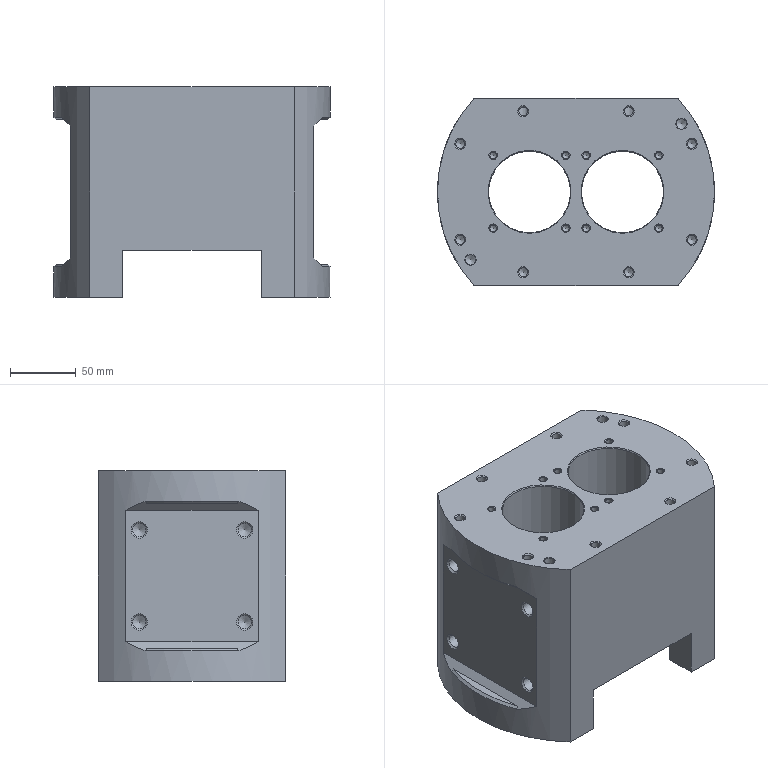NC program | NX | posted with a generic post | part box 210 x 142 x 160 mm
Lines 1 to 1156 of 4199:
N10 G17 G21 G94 G90
(FLOOR_WALL_COPY_COPY_COPY_COPY_1_COPY , TOOL : D50)
N12 T02 M6
N14 G54
N16 G17 G0 G90 X-133. Y70.997 B0. C0. S2500 M3
N18 G43 Z30. H2
N20 Z3.
N22 G94 G1 Z0. F1000.
N24 X-130.
N26 X130.
N28 Y40.498
N30 X-130.
N32 Y9.999
N34 X130.
N36 Y-20.501
N38 X-130.
N40 Y-51.
N42 X130.
N44 X133.
N46 Z3.
N48 G0 Z30.
(FLOOR_WALL_1 , TOOL : D50)
N50 X3.83 Y-99. S1200
N52 Z0.652
N54 G1 Z-0.348
N56 Y-72.786
N58 G3 X0. Y-71. R5.
N60 G1 X-27.35 F2000.
N62 Y-30.308
N64 X-43.993 Y-24.326
N66 G2 X-43.993 Y24.326 R25.85
N68 G1 X-33.127 Y28.232
N70 X-27.35 Y30.308
N72 Y71.
N74 X27.35
N76 Y30.308
N78 X43.993 Y24.326
N80 G2 X43.993 Y-24.326 R25.85
N82 G1 X33.127 Y-28.232
N84 X27.35 Y-30.308
N86 Y-71.
N88 X0.
N90 Y-17.98
N92 G3 X-17.203 Y-2.077 R30.
N94 G1 X-22.98 Y0.
N96 X-17.204 Y2.076
N98 G3 X0. Y17.98 R30.
N100 G1 Y44.472
N102 Y17.98
N104 G3 X17.203 Y2.077 R30.
N106 G1 X22.98 Y0.
N108 X17.203 Y-2.077
N110 G3 X0. Y-17.98 R30.
N112 X0.054 Y-22.206 R5.
N114 G1 Z0.652
N116 G0 X3.83 Y-99. Z0.304
N118 G1 Z-0.696 F1000.
N120 Y-72.786
N122 G3 X0. Y-71. R5.
N124 G1 X-27.35 F2000.
N126 Y-30.308
N128 X-43.993 Y-24.326
N130 G2 X-43.993 Y24.326 R25.85
N132 G1 X-33.127 Y28.232
N134 X-27.35 Y30.308
N136 Y71.
N138 X27.35
N140 Y30.308
N142 X43.993 Y24.326
N144 G2 X43.993 Y-24.326 R25.85
N146 G1 X33.127 Y-28.232
N148 X27.35 Y-30.308
N150 Y-71.
N152 X0.
N154 Y-17.98
N156 G3 X-17.203 Y-2.077 R30.
N158 G1 X-22.98 Y0.
N160 X-17.204 Y2.076
N162 G3 X0. Y17.98 R30.
N164 G1 Y44.472
N166 Y17.98
N168 G3 X17.203 Y2.077 R30.
N170 G1 X22.98 Y0.
N172 X17.203 Y-2.077
N174 G3 X0. Y-17.98 R30.
N176 X0.054 Y-22.206 R5.
N178 G1 Z0.304
N180 G0 X3.83 Y-99. Z-0.044
N182 G1 Z-1.044 F1000.
N184 Y-72.786
N186 G3 X0. Y-71. R5.
N188 G1 X-27.35 F2000.
N190 Y-30.308
N192 X-43.993 Y-24.326
N194 G2 X-43.993 Y24.326 R25.85
N196 G1 X-33.127 Y28.232
N198 X-27.35 Y30.308
N200 Y71.
N202 X27.35
N204 Y30.308
N206 X43.993 Y24.326
N208 G2 X43.993 Y-24.326 R25.85
N210 G1 X33.127 Y-28.232
N212 X27.35 Y-30.308
N214 Y-71.
N216 X0.
N218 Y-17.98
N220 G3 X-17.203 Y-2.077 R30.
N222 G1 X-22.98 Y0.
N224 X-17.204 Y2.076
N226 G3 X0. Y17.98 R30.
N228 G1 Y44.472
N230 Y17.98
N232 G3 X17.203 Y2.077 R30.
N234 G1 X22.98 Y0.
N236 X17.203 Y-2.077
N238 G3 X0. Y-17.98 R30.
N240 X0.054 Y-22.206 R5.
N242 G1 Z-0.044
N244 G0 X3.83 Y-99. Z-0.392
N246 G1 Z-1.392 F1000.
N248 Y-72.786
N250 G3 X0. Y-71. R5.
N252 G1 X-27.35 F2000.
N254 Y-30.308
N256 X-43.993 Y-24.326
N258 G2 X-43.993 Y24.326 R25.85
N260 G1 X-33.127 Y28.232
N262 X-27.35 Y30.308
N264 Y71.
N266 X27.35
N268 Y30.308
N270 X43.993 Y24.326
N272 G2 X43.993 Y-24.326 R25.85
N274 G1 X33.127 Y-28.232
N276 X27.35 Y-30.308
N278 Y-71.
N280 X0.
N282 Y-17.98
N284 G3 X-17.203 Y-2.077 R30.
N286 G1 X-22.98 Y0.
N288 X-17.204 Y2.076
N290 G3 X0. Y17.98 R30.
N292 G1 Y44.472
N294 Y17.98
N296 G3 X17.203 Y2.077 R30.
N298 G1 X22.98 Y0.
N300 X17.203 Y-2.077
N302 G3 X0. Y-17.98 R30.
N304 X0.054 Y-22.206 R5.
N306 G1 Z-0.392
N308 G0 X3.83 Y-99. Z-0.74
N310 G1 Z-1.74 F1000.
N312 Y-72.786
N314 G3 X0. Y-71. R5.
N316 G1 X-27.35 F2000.
N318 Y-30.308
N320 X-43.993 Y-24.326
N322 G2 X-43.993 Y24.326 R25.85
N324 G1 X-33.127 Y28.232
N326 X-27.35 Y30.308
N328 Y71.
N330 X27.35
N332 Y30.308
N334 X43.993 Y24.326
N336 G2 X43.993 Y-24.326 R25.85
N338 G1 X33.127 Y-28.232
N340 X27.35 Y-30.308
N342 Y-71.
N344 X0.
N346 Y-17.98
N348 G3 X-17.203 Y-2.077 R30.
N350 G1 X-22.98 Y0.
N352 X-17.204 Y2.076
N354 G3 X0. Y17.98 R30.
N356 G1 Y44.472
N358 Y17.98
N360 G3 X17.203 Y2.077 R30.
N362 G1 X22.98 Y0.
N364 X17.203 Y-2.077
N366 G3 X0. Y-17.98 R30.
N368 X0.054 Y-22.206 R5.
N370 G1 Z-0.74
N372 G0 X3.83 Y-99. Z-1.088
N374 G1 Z-2.088 F1000.
N376 Y-72.786
N378 G3 X0. Y-71. R5.
N380 G1 X-27.35 F2000.
N382 Y-30.308
N384 X-43.993 Y-24.326
N386 G2 X-43.993 Y24.326 R25.85
N388 G1 X-33.127 Y28.232
N390 X-27.35 Y30.308
N392 Y71.
N394 X27.35
N396 Y30.308
N398 X43.993 Y24.326
N400 G2 X43.993 Y-24.326 R25.85
N402 G1 X33.127 Y-28.232
N404 X27.35 Y-30.308
N406 Y-71.
N408 X0.
N410 Y-17.98
N412 G3 X-17.203 Y-2.077 R30.
N414 G1 X-22.98 Y0.
N416 X-17.204 Y2.076
N418 G3 X0. Y17.98 R30.
N420 G1 Y44.472
N422 Y17.98
N424 G3 X17.203 Y2.077 R30.
N426 G1 X22.98 Y0.
N428 X17.203 Y-2.077
N430 G3 X0. Y-17.98 R30.
N432 X0.054 Y-22.206 R5.
N434 G1 Z-1.088
N436 G0 X3.83 Y-99. Z-1.436
N438 G1 Z-2.436 F1000.
N440 Y-72.786
N442 G3 X0. Y-71. R5.
N444 G1 X-27.35 F2000.
N446 Y-30.308
N448 X-43.993 Y-24.326
N450 G2 X-43.993 Y24.326 R25.85
N452 G1 X-33.127 Y28.232
N454 X-27.35 Y30.308
N456 Y71.
N458 X27.35
N460 Y30.308
N462 X43.993 Y24.326
N464 G2 X43.993 Y-24.326 R25.85
N466 G1 X33.127 Y-28.232
N468 X27.35 Y-30.308
N470 Y-71.
N472 X0.
N474 Y-17.98
N476 G3 X-17.203 Y-2.077 R30.
N478 G1 X-22.98 Y0.
N480 X-17.204 Y2.076
N482 G3 X0. Y17.98 R30.
N484 G1 Y44.472
N486 Y17.98
N488 G3 X17.203 Y2.077 R30.
N490 G1 X22.98 Y0.
N492 X17.203 Y-2.077
N494 G3 X0. Y-17.98 R30.
N496 X0.054 Y-22.206 R5.
N498 G1 Z-1.436
N500 G0 X3.83 Y-99. Z-1.784
N502 G1 Z-2.784 F1000.
N504 Y-72.786
N506 G3 X0. Y-71. R5.
N508 G1 X-27.35 F2000.
N510 Y-30.308
N512 X-43.993 Y-24.326
N514 G2 X-43.993 Y24.326 R25.85
N516 G1 X-33.127 Y28.232
N518 X-27.35 Y30.308
N520 Y71.
N522 X27.35
N524 Y30.308
N526 X43.993 Y24.326
N528 G2 X43.993 Y-24.326 R25.85
N530 G1 X33.127 Y-28.232
N532 X27.35 Y-30.308
N534 Y-71.
N536 X0.
N538 Y-17.98
N540 G3 X-17.203 Y-2.077 R30.
N542 G1 X-22.98 Y0.
N544 X-17.204 Y2.076
N546 G3 X0. Y17.98 R30.
N548 G1 Y44.472
N550 Y17.98
N552 G3 X17.203 Y2.077 R30.
N554 G1 X22.98 Y0.
N556 X17.203 Y-2.077
N558 G3 X0. Y-17.98 R30.
N560 X0.054 Y-22.206 R5.
N562 G1 Z-1.784
N564 G0 X3.83 Y-99. Z-2.133
N566 G1 Z-3.133 F1000.
N568 Y-72.786
N570 G3 X0. Y-71. R5.
N572 G1 X-27.35 F2000.
N574 Y-30.308
N576 X-43.993 Y-24.326
N578 G2 X-43.993 Y24.326 R25.85
N580 G1 X-33.127 Y28.232
N582 X-27.35 Y30.308
N584 Y71.
N586 X27.35
N588 Y30.308
N590 X43.993 Y24.326
N592 G2 X43.993 Y-24.326 R25.85
N594 G1 X33.127 Y-28.232
N596 X27.35 Y-30.308
N598 Y-71.
N600 X0.
N602 Y-17.98
N604 G3 X-17.203 Y-2.077 R30.
N606 G1 X-22.98 Y0.
N608 X-17.204 Y2.076
N610 G3 X0. Y17.98 R30.
N612 G1 Y44.472
N614 Y17.98
N616 G3 X17.203 Y2.077 R30.
N618 G1 X22.98 Y0.
N620 X17.203 Y-2.077
N622 G3 X0. Y-17.98 R30.
N624 X0.054 Y-22.206 R5.
N626 G1 Z-2.133
N628 G0 X3.83 Y-99. Z-2.481
N630 G1 Z-3.481 F1000.
N632 Y-72.786
N634 G3 X0. Y-71. R5.
N636 G1 X-27.35 F2000.
N638 Y-30.308
N640 X-43.993 Y-24.326
N642 G2 X-43.993 Y24.326 R25.85
N644 G1 X-33.127 Y28.232
N646 X-27.35 Y30.308
N648 Y71.
N650 X27.35
N652 Y30.308
N654 X43.993 Y24.326
N656 G2 X43.993 Y-24.326 R25.85
N658 G1 X33.127 Y-28.232
N660 X27.35 Y-30.308
N662 Y-71.
N664 X0.
N666 Y-17.98
N668 G3 X-17.203 Y-2.077 R30.
N670 G1 X-22.98 Y0.
N672 X-17.204 Y2.076
N674 G3 X0. Y17.98 R30.
N676 G1 Y44.472
N678 Y17.98
N680 G3 X17.203 Y2.077 R30.
N682 G1 X22.98 Y0.
N684 X17.203 Y-2.077
N686 G3 X0. Y-17.98 R30.
N688 X0.054 Y-22.206 R5.
N690 G1 Z-2.481
N692 G0 X3.83 Y-99. Z-2.829
N694 G1 Z-3.829 F1000.
N696 Y-72.786
N698 G3 X0. Y-71. R5.
N700 G1 X-27.35 F2000.
N702 Y-30.308
N704 X-43.993 Y-24.326
N706 G2 X-43.993 Y24.326 R25.85
N708 G1 X-33.127 Y28.232
N710 X-27.35 Y30.308
N712 Y71.
N714 X27.35
N716 Y30.308
N718 X43.993 Y24.326
N720 G2 X43.993 Y-24.326 R25.85
N722 G1 X33.127 Y-28.232
N724 X27.35 Y-30.308
N726 Y-71.
N728 X0.
N730 Y-17.98
N732 G3 X-17.203 Y-2.077 R30.
N734 G1 X-22.98 Y0.
N736 X-17.204 Y2.076
N738 G3 X0. Y17.98 R30.
N740 G1 Y44.472
N742 Y17.98
N744 G3 X17.203 Y2.077 R30.
N746 G1 X22.98 Y0.
N748 X17.203 Y-2.077
N750 G3 X0. Y-17.98 R30.
N752 X0.054 Y-22.206 R5.
N754 G1 Z-2.829
N756 G0 X3.83 Y-99. Z-3.177
N758 G1 Z-4.177 F1000.
N760 Y-72.786
N762 G3 X0. Y-71. R5.
N764 G1 X-27.35 F2000.
N766 Y-30.308
N768 X-43.993 Y-24.326
N770 G2 X-43.993 Y24.326 R25.85
N772 G1 X-33.127 Y28.232
N774 X-27.35 Y30.308
N776 Y71.
N778 X27.35
N780 Y30.308
N782 X43.993 Y24.326
N784 G2 X43.993 Y-24.326 R25.85
N786 G1 X33.127 Y-28.232
N788 X27.35 Y-30.308
N790 Y-71.
N792 X0.
N794 Y-17.98
N796 G3 X-17.203 Y-2.077 R30.
N798 G1 X-22.98 Y0.
N800 X-17.204 Y2.076
N802 G3 X0. Y17.98 R30.
N804 G1 Y44.472
N806 Y17.98
N808 G3 X17.203 Y2.077 R30.
N810 G1 X22.98 Y0.
N812 X17.203 Y-2.077
N814 G3 X0. Y-17.98 R30.
N816 X0.054 Y-22.206 R5.
N818 G1 Z-3.177
N820 G0 X3.83 Y-99. Z-3.525
N822 G1 Z-4.525 F1000.
N824 Y-72.786
N826 G3 X0. Y-71. R5.
N828 G1 X-27.35 F2000.
N830 Y-30.308
N832 X-43.993 Y-24.326
N834 G2 X-43.993 Y24.326 R25.85
N836 G1 X-33.127 Y28.232
N838 X-27.35 Y30.308
N840 Y71.
N842 X27.35
N844 Y30.308
N846 X43.993 Y24.326
N848 G2 X43.993 Y-24.326 R25.85
N850 G1 X33.127 Y-28.232
N852 X27.35 Y-30.308
N854 Y-71.
N856 X0.
N858 Y-17.98
N860 G3 X-17.203 Y-2.077 R30.
N862 G1 X-22.98 Y0.
N864 X-17.204 Y2.076
N866 G3 X0. Y17.98 R30.
N868 G1 Y44.472
N870 Y17.98
N872 G3 X17.203 Y2.077 R30.
N874 G1 X22.98 Y0.
N876 X17.203 Y-2.077
N878 G3 X0. Y-17.98 R30.
N880 X0.054 Y-22.206 R5.
N882 G1 Z-3.525
N884 G0 X3.83 Y-99. Z-3.873
N886 G1 Z-4.873 F1000.
N888 Y-72.786
N890 G3 X0. Y-71. R5.
N892 G1 X-27.35 F2000.
N894 Y-30.308
N896 X-43.993 Y-24.326
N898 G2 X-43.993 Y24.326 R25.85
N900 G1 X-33.127 Y28.232
N902 X-27.35 Y30.308
N904 Y71.
N906 X27.35
N908 Y30.308
N910 X43.993 Y24.326
N912 G2 X43.993 Y-24.326 R25.85
N914 G1 X33.127 Y-28.232
N916 X27.35 Y-30.308
N918 Y-71.
N920 X0.
N922 Y-17.98
N924 G3 X-17.203 Y-2.077 R30.
N926 G1 X-22.98 Y0.
N928 X-17.204 Y2.076
N930 G3 X0. Y17.98 R30.
N932 G1 Y44.472
N934 Y17.98
N936 G3 X17.203 Y2.077 R30.
N938 G1 X22.98 Y0.
N940 X17.203 Y-2.077
N942 G3 X0. Y-17.98 R30.
N944 X0.054 Y-22.206 R5.
N946 G1 Z-3.873
N948 G0 X3.83 Y-99. Z-4.221
N950 G1 Z-5.221 F1000.
N952 Y-72.786
N954 G3 X0. Y-71. R5.
N956 G1 X-27.35 F2000.
N958 Y-30.308
N960 X-43.993 Y-24.326
N962 G2 X-43.993 Y24.326 R25.85
N964 G1 X-33.127 Y28.232
N966 X-27.35 Y30.308
N968 Y71.
N970 X27.35
N972 Y30.308
N974 X43.993 Y24.326
N976 G2 X43.993 Y-24.326 R25.85
N978 G1 X33.127 Y-28.232
N980 X27.35 Y-30.308
N982 Y-71.
N984 X0.
N986 Y-17.98
N988 G3 X-17.203 Y-2.077 R30.
N990 G1 X-22.98 Y0.
N992 X-17.204 Y2.076
N994 G3 X0. Y17.98 R30.
N996 G1 Y44.472
N998 Y17.98
N1000 G3 X17.203 Y2.077 R30.
N1002 G1 X22.98 Y0.
N1004 X17.203 Y-2.077
N1006 G3 X0. Y-17.98 R30.
N1008 X0.054 Y-22.206 R5.
N1010 G1 Z-4.221
N1012 G0 X3.83 Y-99. Z-4.569
N1014 G1 Z-5.569 F1000.
N1016 Y-72.786
N1018 G3 X0. Y-71. R5.
N1020 G1 X-27.35 F2000.
N1022 Y-30.308
N1024 X-43.993 Y-24.326
N1026 G2 X-43.993 Y24.326 R25.85
N1028 G1 X-33.127 Y28.232
N1030 X-27.35 Y30.308
N1032 Y71.
N1034 X27.35
N1036 Y30.308
N1038 X43.993 Y24.326
N1040 G2 X43.993 Y-24.326 R25.85
N1042 G1 X33.127 Y-28.232
N1044 X27.35 Y-30.308
N1046 Y-71.
N1048 X0.
N1050 Y-17.98
N1052 G3 X-17.203 Y-2.077 R30.
N1054 G1 X-22.98 Y0.
N1056 X-17.204 Y2.076
N1058 G3 X0. Y17.98 R30.
N1060 G1 Y44.472
N1062 Y17.98
N1064 G3 X17.203 Y2.077 R30.
N1066 G1 X22.98 Y0.
N1068 X17.203 Y-2.077
N1070 G3 X0. Y-17.98 R30.
N1072 X0.054 Y-22.206 R5.
N1074 G1 Z-4.569
N1076 G0 X3.83 Y-99. Z-4.917
N1078 G1 Z-5.917 F1000.
N1080 Y-72.786
N1082 G3 X0. Y-71. R5.
N1084 G1 X-27.35 F2000.
N1086 Y-30.308
N1088 X-43.993 Y-24.326
N1090 G2 X-43.993 Y24.326 R25.85
N1092 G1 X-33.127 Y28.232
N1094 X-27.35 Y30.308
N1096 Y71.
N1098 X27.35
N1100 Y30.308
N1102 X43.993 Y24.326
N1104 G2 X43.993 Y-24.326 R25.85
N1106 G1 X33.127 Y-28.232
N1108 X27.35 Y-30.308
N1110 Y-71.
N1112 X0.
N1114 Y-17.98
N1116 G3 X-17.203 Y-2.077 R30.
N1118 G1 X-22.98 Y0.
N1120 X-17.204 Y2.076
N1122 G3 X0. Y17.98 R30.
N1124 G1 Y44.472
N1126 Y17.98
N1128 G3 X17.203 Y2.077 R30.
N1130 G1 X22.98 Y0.
N1132 X17.203 Y-2.077
N1134 G3 X0. Y-17.98 R30.
N1136 X0.054 Y-22.206 R5.
N1138 G1 Z-4.917
N1140 G0 X3.83 Y-99. Z-5.265
N1142 G1 Z-6.265 F1000.
N1144 Y-72.786
N1146 G3 X0. Y-71. R5.
N1148 G1 X-27.35 F2000.
N1150 Y-30.308
N1152 X-43.993 Y-24.326
N1154 G2 X-43.993 Y24.326 R25.85
N1156 G1 X-33.127 Y28.232
N1158 X-27.35 Y30.308
N1160 Y71.
N1162 X27.35
N1164 Y30.308
N1166 X43.993 Y24.326
N1168 G2 X43.993 Y-24.326 R25.85
N1170 G1 X33.127 Y-28.232
N1172 X27.35 Y-30.308
N1174 Y-71.
N1176 X0.
N1178 Y-17.98
N1180 G3 X-17.203 Y-2.077 R30.
N1182 G1 X-22.98 Y0.
N1184 X-17.204 Y2.076
N1186 G3 X0. Y17.98 R30.
N1188 G1 Y44.472
N1190 Y17.98
N1192 G3 X17.203 Y2.077 R30.
N1194 G1 X22.98 Y0.
N1196 X17.203 Y-2.077
N1198 G3 X0. Y-17.98 R30.
N1200 X0.054 Y-22.206 R5.
N1202 G1 Z-5.265
N1204 G0 X3.83 Y-99. Z-5.613
N1206 G1 Z-6.613 F1000.
N1208 Y-72.786
N1210 G3 X0. Y-71. R5.
N1212 G1 X-27.35 F2000.
N1214 Y-30.308
N1216 X-43.993 Y-24.326
N1218 G2 X-43.993 Y24.326 R25.85
N1220 G1 X-33.127 Y28.232
N1222 X-27.35 Y30.308
N1224 Y71.
N1226 X27.35
N1228 Y30.308
N1230 X43.993 Y24.326
N1232 G2 X43.993 Y-24.326 R25.85
N1234 G1 X33.127 Y-28.232
N1236 X27.35 Y-30.308
N1238 Y-71.
N1240 X0.
N1242 Y-17.98
N1244 G3 X-17.203 Y-2.077 R30.
N1246 G1 X-22.98 Y0.
N1248 X-17.204 Y2.076
N1250 G3 X0. Y17.98 R30.
N1252 G1 Y44.472
N1254 Y17.98
N1256 G3 X17.203 Y2.077 R30.
N1258 G1 X22.98 Y0.
N1260 X17.203 Y-2.077
N1262 G3 X0. Y-17.98 R30.
N1264 X0.054 Y-22.206 R5.
N1266 G1 Z-5.613
N1268 G0 X3.83 Y-99. Z-5.961
N1270 G1 Z-6.961 F1000.
N1272 Y-72.786
N1274 G3 X0. Y-71. R5.
N1276 G1 X-27.35 F2000.
N1278 Y-30.308
N1280 X-43.993 Y-24.326
N1282 G2 X-43.993 Y24.326 R25.85
N1284 G1 X-33.127 Y28.232
N1286 X-27.35 Y30.308
N1288 Y71.
N1290 X27.35
N1292 Y30.308
N1294 X43.993 Y24.326
N1296 G2 X43.993 Y-24.326 R25.85
N1298 G1 X33.127 Y-28.232
N1300 X27.35 Y-30.308
N1302 Y-71.
N1304 X0.
N1306 Y-17.98
N1308 G3 X-17.203 Y-2.077 R30.
N1310 G1 X-22.98 Y0.
N1312 X-17.204 Y2.076
N1314 G3 X0. Y17.98 R30.
N1316 G1 Y44.472
N1318 Y17.98
N1320 G3 X17.203 Y2.077 R30.
N1322 G1 X22.98 Y0.
N1324 X17.203 Y-2.077
N1326 G3 X0. Y-17.98 R30.
N1328 X0.054 Y-22.206 R5.
N1330 G1 Z-5.961
N1332 G0 X3.83 Y-99. Z-6.309
N1334 G1 Z-7.309 F1000.
N1336 Y-72.786
N1338 G3 X0. Y-71. R5.
N1340 G1 X-27.35 F2000.
N1342 Y-30.308
N1344 X-43.993 Y-24.326
N1346 G2 X-43.993 Y24.326 R25.85
N1348 G1 X-33.127 Y28.232
N1350 X-27.35 Y30.308
N1352 Y71.
N1354 X27.35
N1356 Y30.308
N1358 X43.993 Y24.326
N1360 G2 X43.993 Y-24.326 R25.85
N1362 G1 X33.127 Y-28.232
N1364 X27.35 Y-30.308
N1366 Y-71.
N1368 X0.
N1370 Y-17.98
N1372 G3 X-17.203 Y-2.077 R30.
N1374 G1 X-22.98 Y0.
N1376 X-17.204 Y2.076
N1378 G3 X0. Y17.98 R30.
N1380 G1 Y44.472
N1382 Y17.98
N1384 G3 X17.203 Y2.077 R30.
N1386 G1 X22.98 Y0.
N1388 X17.203 Y-2.077
N1390 G3 X0. Y-17.98 R30.
N1392 X0.054 Y-22.206 R5.
N1394 G1 Z-6.309
N1396 G0 X3.83 Y-99. Z-6.657
N1398 G1 Z-7.657 F1000.
N1400 Y-72.786
N1402 G3 X0. Y-71. R5.
N1404 G1 X-27.35 F2000.
N1406 Y-30.308
N1408 X-43.993 Y-24.326
N1410 G2 X-43.993 Y24.326 R25.85
N1412 G1 X-33.127 Y28.232
N1414 X-27.35 Y30.308
N1416 Y71.
N1418 X27.35
N1420 Y30.308
N1422 X43.993 Y24.326
N1424 G2 X43.993 Y-24.326 R25.85
N1426 G1 X33.127 Y-28.232
N1428 X27.35 Y-30.308
N1430 Y-71.
N1432 X0.
N1434 Y-17.98
N1436 G3 X-17.203 Y-2.077 R30.
N1438 G1 X-22.98 Y0.
N1440 X-17.204 Y2.076
N1442 G3 X0. Y17.98 R30.
N1444 G1 Y44.472
N1446 Y17.98
N1448 G3 X17.203 Y2.077 R30.
N1450 G1 X22.98 Y0.
N1452 X17.203 Y-2.077
N1454 G3 X0. Y-17.98 R30.
N1456 X0.054 Y-22.206 R5.
N1458 G1 Z-6.657
N1460 G0 X3.83 Y-99. Z-7.005
N1462 G1 Z-8.005 F1000.
N1464 Y-72.786
N1466 G3 X0. Y-71. R5.
N1468 G1 X-27.35 F2000.
N1470 Y-30.308
N1472 X-43.993 Y-24.326
N1474 G2 X-43.993 Y24.326 R25.85
N1476 G1 X-33.127 Y28.232
N1478 X-27.35 Y30.308
N1480 Y71.
N1482 X27.35
N1484 Y30.308
N1486 X43.993 Y24.326
N1488 G2 X43.993 Y-24.326 R25.85
N1490 G1 X33.127 Y-28.232
N1492 X27.35 Y-30.308
N1494 Y-71.
N1496 X0.
N1498 Y-17.98
N1500 G3 X-17.203 Y-2.077 R30.
N1502 G1 X-22.98 Y0.
N1504 X-17.204 Y2.076
N1506 G3 X0. Y17.98 R30.
N1508 G1 Y44.472
N1510 Y17.98
N1512 G3 X17.203 Y2.077 R30.
N1514 G1 X22.98 Y0.
N1516 X17.203 Y-2.077
N1518 G3 X0. Y-17.98 R30.
N1520 X0.054 Y-22.206 R5.
N1522 G1 Z-7.005
N1524 G0 X3.83 Y-99. Z-7.353
N1526 G1 Z-8.353 F1000.
N1528 Y-72.786
N1530 G3 X0. Y-71. R5.
N1532 G1 X-27.35 F2000.
N1534 Y-30.308
N1536 X-43.993 Y-24.326
N1538 G2 X-43.993 Y24.326 R25.85
N1540 G1 X-33.127 Y28.232
N1542 X-27.35 Y30.308
N1544 Y71.
N1546 X27.35
N1548 Y30.308
N1550 X43.993 Y24.326
N1552 G2 X43.993 Y-24.326 R25.85
N1554 G1 X33.127 Y-28.232
N1556 X27.35 Y-30.308
N1558 Y-71.
N1560 X0.
N1562 Y-17.98
N1564 G3 X-17.203 Y-2.077 R30.
N1566 G1 X-22.98 Y0.
N1568 X-17.204 Y2.076
N1570 G3 X0. Y17.98 R30.
N1572 G1 Y44.472
N1574 Y17.98
N1576 G3 X17.203 Y2.077 R30.
N1578 G1 X22.98 Y0.
N1580 X17.203 Y-2.077
N1582 G3 X0. Y-17.98 R30.
N1584 X0.054 Y-22.206 R5.
N1586 G1 Z-7.353
N1588 G0 X3.83 Y-99. Z-7.701
N1590 G1 Z-8.701 F1000.
N1592 Y-72.786
N1594 G3 X0. Y-71. R5.
N1596 G1 X-27.35 F2000.
N1598 Y-30.308
N1600 X-43.993 Y-24.326
N1602 G2 X-43.993 Y24.326 R25.85
N1604 G1 X-33.127 Y28.232
N1606 X-27.35 Y30.308
N1608 Y71.
N1610 X27.35
N1612 Y30.308
N1614 X43.993 Y24.326
N1616 G2 X43.993 Y-24.326 R25.85
N1618 G1 X33.127 Y-28.232
N1620 X27.35 Y-30.308
N1622 Y-71.
N1624 X0.
N1626 Y-17.98
N1628 G3 X-17.203 Y-2.077 R30.
N1630 G1 X-22.98 Y0.
N1632 X-17.204 Y2.076
N1634 G3 X0. Y17.98 R30.
N1636 G1 Y44.472
N1638 Y17.98
N1640 G3 X17.203 Y2.077 R30.
N1642 G1 X22.98 Y0.
N1644 X17.203 Y-2.077
N1646 G3 X0. Y-17.98 R30.
N1648 X0.054 Y-22.206 R5.
N1650 G1 Z-7.701
N1652 G0 X3.83 Y-99. Z-8.05
N1654 G1 Z-9.05 F1000.
N1656 Y-72.786
N1658 G3 X0. Y-71. R5.
N1660 G1 X-27.35 F2000.
N1662 Y-30.308
N1664 X-43.993 Y-24.326
N1666 G2 X-43.993 Y24.326 R25.85
N1668 G1 X-33.127 Y28.232
N1670 X-27.35 Y30.308
N1672 Y71.
N1674 X27.35
N1676 Y30.308
N1678 X43.993 Y24.326
N1680 G2 X43.993 Y-24.326 R25.85
N1682 G1 X33.127 Y-28.232
N1684 X27.35 Y-30.308
N1686 Y-71.
N1688 X0.
N1690 Y-17.98
N1692 G3 X-17.203 Y-2.077 R30.
N1694 G1 X-22.98 Y0.
N1696 X-17.204 Y2.076
N1698 G3 X0. Y17.98 R30.
N1700 G1 Y44.472
N1702 Y17.98
N1704 G3 X17.203 Y2.077 R30.
N1706 G1 X22.98 Y0.
N1708 X17.203 Y-2.077
N1710 G3 X0. Y-17.98 R30.
N1712 X0.054 Y-22.206 R5.
N1714 G1 Z-8.05
N1716 G0 X3.83 Y-99. Z-8.398
N1718 G1 Z-9.398 F1000.
N1720 Y-72.786
N1722 G3 X0. Y-71. R5.
N1724 G1 X-27.35 F2000.
N1726 Y-30.308
N1728 X-43.993 Y-24.326
N1730 G2 X-43.993 Y24.326 R25.85
N1732 G1 X-33.127 Y28.232
N1734 X-27.35 Y30.308
N1736 Y71.
N1738 X27.35
N1740 Y30.308
N1742 X43.993 Y24.326
N1744 G2 X43.993 Y-24.326 R25.85
N1746 G1 X33.127 Y-28.232
N1748 X27.35 Y-30.308
N1750 Y-71.
N1752 X0.
N1754 Y-17.98
N1756 G3 X-17.203 Y-2.077 R30.
N1758 G1 X-22.98 Y0.
N1760 X-17.204 Y2.076
N1762 G3 X0. Y17.98 R30.
N1764 G1 Y44.472
N1766 Y17.98
N1768 G3 X17.203 Y2.077 R30.
N1770 G1 X22.98 Y0.
N1772 X17.203 Y-2.077
N1774 G3 X0. Y-17.98 R30.
N1776 X0.054 Y-22.206 R5.
N1778 G1 Z-8.398
N1780 G0 X3.83 Y-99. Z-8.746
N1782 G1 Z-9.746 F1000.
N1784 Y-72.786
N1786 G3 X0. Y-71. R5.
N1788 G1 X-27.35 F2000.
N1790 Y-30.308
N1792 X-43.993 Y-24.326
N1794 G2 X-43.993 Y24.326 R25.85
N1796 G1 X-33.127 Y28.232
N1798 X-27.35 Y30.308
N1800 Y71.
N1802 X27.35
N1804 Y30.308
N1806 X43.993 Y24.326
N1808 G2 X43.993 Y-24.326 R25.85
N1810 G1 X33.127 Y-28.232
N1812 X27.35 Y-30.308
N1814 Y-71.
N1816 X0.
N1818 Y-17.98
N1820 G3 X-17.203 Y-2.077 R30.
N1822 G1 X-22.98 Y0.
N1824 X-17.204 Y2.076
N1826 G3 X0. Y17.98 R30.
N1828 G1 Y44.472
N1830 Y17.98
N1832 G3 X17.203 Y2.077 R30.
N1834 G1 X22.98 Y0.
N1836 X17.203 Y-2.077
N1838 G3 X0. Y-17.98 R30.
N1840 X0.054 Y-22.206 R5.
N1842 G1 Z-8.746
N1844 G0 X3.83 Y-99. Z-9.094
N1846 G1 Z-10.094 F1000.
N1848 Y-72.786
N1850 G3 X0. Y-71. R5.
N1852 G1 X-27.35 F2000.
N1854 Y-30.308
N1856 X-43.993 Y-24.326
N1858 G2 X-43.993 Y24.326 R25.85
N1860 G1 X-33.127 Y28.232
N1862 X-27.35 Y30.308
N1864 Y71.
N1866 X27.35
N1868 Y30.308
N1870 X43.993 Y24.326
N1872 G2 X43.993 Y-24.326 R25.85
N1874 G1 X33.127 Y-28.232
N1876 X27.35 Y-30.308
N1878 Y-71.
N1880 X0.
N1882 Y-17.98
N1884 G3 X-17.203 Y-2.077 R30.
N1886 G1 X-22.98 Y0.
N1888 X-17.204 Y2.076
N1890 G3 X0. Y17.98 R30.
N1892 G1 Y44.472
N1894 Y17.98
N1896 G3 X17.203 Y2.077 R30.
N1898 G1 X22.98 Y0.
N1900 X17.203 Y-2.077
N1902 G3 X0. Y-17.98 R30.
N1904 X0.054 Y-22.206 R5.
N1906 G1 Z-9.094
N1908 G0 X3.83 Y-99. Z-9.442
N1910 G1 Z-10.442 F1000.
N1912 Y-72.786
N1914 G3 X0. Y-71. R5.
N1916 G1 X-27.35 F2000.
N1918 Y-30.308
N1920 X-43.993 Y-24.326
N1922 G2 X-43.993 Y24.326 R25.85
N1924 G1 X-33.127 Y28.232
N1926 X-27.35 Y30.308
N1928 Y71.
N1930 X27.35
N1932 Y30.308
N1934 X43.993 Y24.326
N1936 G2 X43.993 Y-24.326 R25.85
N1938 G1 X33.127 Y-28.232
N1940 X27.35 Y-30.308
N1942 Y-71.
N1944 X0.
N1946 Y-17.98
N1948 G3 X-17.203 Y-2.077 R30.
N1950 G1 X-22.98 Y0.
N1952 X-17.204 Y2.076
N1954 G3 X0. Y17.98 R30.
N1956 G1 Y44.472
N1958 Y17.98
N1960 G3 X17.203 Y2.077 R30.
N1962 G1 X22.98 Y0.
N1964 X17.203 Y-2.077
N1966 G3 X0. Y-17.98 R30.
N1968 X0.054 Y-22.206 R5.
N1970 G1 Z-9.442
N1972 G0 X3.83 Y-99. Z-9.79
N1974 G1 Z-10.79 F1000.
N1976 Y-72.786
N1978 G3 X0. Y-71. R5.
N1980 G1 X-27.35 F2000.
N1982 Y-30.308
N1984 X-43.993 Y-24.326
N1986 G2 X-43.993 Y24.326 R25.85
N1988 G1 X-33.127 Y28.232
N1990 X-27.35 Y30.308
N1992 Y71.
N1994 X27.35
N1996 Y30.308
N1998 X43.993 Y24.326
N2000 G2 X43.993 Y-24.326 R25.85
N2002 G1 X33.127 Y-28.232
N2004 X27.35 Y-30.308
N2006 Y-71.
N2008 X0.
N2010 Y-17.98
N2012 G3 X-17.203 Y-2.077 R30.
N2014 G1 X-22.98 Y0.
N2016 X-17.204 Y2.076
N2018 G3 X0. Y17.98 R30.
N2020 G1 Y44.472
N2022 Y17.98
N2024 G3 X17.203 Y2.077 R30.
N2026 G1 X22.98 Y0.
N2028 X17.203 Y-2.077
N2030 G3 X0. Y-17.98 R30.
N2032 X0.054 Y-22.206 R5.
N2034 G1 Z-9.79
N2036 G0 X3.83 Y-99. Z-10.138
N2038 G1 Z-11.138 F1000.
N2040 Y-72.786
N2042 G3 X0. Y-71. R5.
N2044 G1 X-27.35 F2000.
N2046 Y-30.308
N2048 X-43.993 Y-24.326
N2050 G2 X-43.993 Y24.326 R25.85
N2052 G1 X-33.127 Y28.232
N2054 X-27.35 Y30.308
N2056 Y71.
N2058 X27.35
N2060 Y30.308
N2062 X43.993 Y24.326
N2064 G2 X43.993 Y-24.326 R25.85
N2066 G1 X33.127 Y-28.232
N2068 X27.35 Y-30.308
N2070 Y-71.
N2072 X0.
N2074 Y-17.98
N2076 G3 X-17.203 Y-2.077 R30.
N2078 G1 X-22.98 Y0.
N2080 X-17.204 Y2.076
N2082 G3 X0. Y17.98 R30.
N2084 G1 Y44.472
N2086 Y17.98
N2088 G3 X17.203 Y2.077 R30.
N2090 G1 X22.98 Y0.
N2092 X17.203 Y-2.077
N2094 G3 X0. Y-17.98 R30.
N2096 X0.054 Y-22.206 R5.
N2098 G1 Z-10.138
N2100 G0 X3.83 Y-99. Z-10.486
N2102 G1 Z-11.486 F1000.
N2104 Y-72.786
N2106 G3 X0. Y-71. R5.
N2108 G1 X-27.35 F2000.
N2110 Y-30.308
N2112 X-43.993 Y-24.326
N2114 G2 X-43.993 Y24.326 R25.85
N2116 G1 X-33.127 Y28.232
N2118 X-27.35 Y30.308
N2120 Y71.
N2122 X27.35
N2124 Y30.308
N2126 X43.993 Y24.326
N2128 G2 X43.993 Y-24.326 R25.85
N2130 G1 X33.127 Y-28.232
N2132 X27.35 Y-30.308
N2134 Y-71.
N2136 X0.
N2138 Y-17.98
N2140 G3 X-17.203 Y-2.077 R30.
N2142 G1 X-22.98 Y0.
N2144 X-17.204 Y2.076
N2146 G3 X0. Y17.98 R30.
N2148 G1 Y44.472
N2150 Y17.98
N2152 G3 X17.203 Y2.077 R30.
N2154 G1 X22.98 Y0.
N2156 X17.203 Y-2.077
N2158 G3 X0. Y-17.98 R30.
N2160 X0.054 Y-22.206 R5.
N2162 G1 Z-10.486
N2164 G0 X3.83 Y-99. Z-10.834
N2166 G1 Z-11.834 F1000.
N2168 Y-72.786
N2170 G3 X0. Y-71. R5.
N2172 G1 X-27.35 F2000.
N2174 Y-30.308
N2176 X-43.993 Y-24.326
N2178 G2 X-43.993 Y24.326 R25.85
N2180 G1 X-33.127 Y28.232
N2182 X-27.35 Y30.308
N2184 Y71.
N2186 X27.35
N2188 Y30.308
N2190 X43.993 Y24.326
N2192 G2 X43.993 Y-24.326 R25.85
N2194 G1 X33.127 Y-28.232
N2196 X27.35 Y-30.308
N2198 Y-71.
N2200 X0.
N2202 Y-17.98
N2204 G3 X-17.203 Y-2.077 R30.
N2206 G1 X-22.98 Y0.
N2208 X-17.204 Y2.076
N2210 G3 X0. Y17.98 R30.
N2212 G1 Y44.472
N2214 Y17.98
N2216 G3 X17.203 Y2.077 R30.
N2218 G1 X22.98 Y0.
N2220 X17.203 Y-2.077
N2222 G3 X0. Y-17.98 R30.
N2224 X0.054 Y-22.206 R5.
N2226 G1 Z-10.834
N2228 G0 X3.83 Y-99. Z-11.182
N2230 G1 Z-12.182 F1000.
N2232 Y-72.786
N2234 G3 X0. Y-71. R5.
N2236 G1 X-27.35 F2000.
N2238 Y-30.308
N2240 X-43.993 Y-24.326
N2242 G2 X-43.993 Y24.326 R25.85
N2244 G1 X-33.127 Y28.232
N2246 X-27.35 Y30.308
N2248 Y71.
N2250 X27.35
N2252 Y30.308
N2254 X43.993 Y24.326
N2256 G2 X43.993 Y-24.326 R25.85
N2258 G1 X33.127 Y-28.232
N2260 X27.35 Y-30.308
N2262 Y-71.
N2264 X0.
N2266 Y-17.98
N2268 G3 X-17.203 Y-2.077 R30.
N2270 G1 X-22.98 Y0.
N2272 X-17.204 Y2.076
N2274 G3 X0. Y17.98 R30.
N2276 G1 Y44.472
N2278 Y17.98
N2280 G3 X17.203 Y2.077 R30.
N2282 G1 X22.98 Y0.
N2284 X17.203 Y-2.077
N2286 G3 X0. Y-17.98 R30.
N2288 X0.054 Y-22.206 R5.
N2290 G1 Z-11.182
N2292 G0 X3.83 Y-99. Z-11.53
N2294 G1 Z-12.53 F1000.
N2296 Y-72.786
N2298 G3 X0. Y-71. R5.
N2300 G1 X-27.35 F2000.
N2302 Y-30.308
N2304 X-43.993 Y-24.326